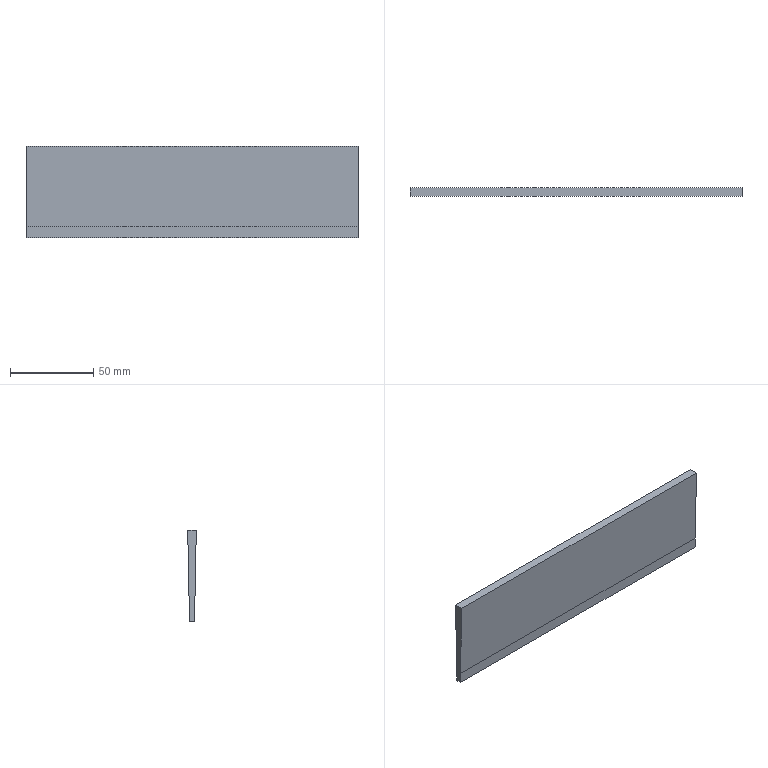Part | NX | features solid 2 | 1 solid | 8 faces | box 200 x 5.155 x 55.03 mm | volume 45049 mm3 | plane 8
STEP:
#1=CARTESIAN_POINT('',(-255.,2183.93,-987.43));
#2=VERTEX_POINT('',#1);
#3=CARTESIAN_POINT('',(-255.,2183.93,-980.8));
#4=VERTEX_POINT('',#3);
#5=CARTESIAN_POINT('',(-255.,2183.93,-987.43));
#6=DIRECTION('',(0.,0.,1.));
#7=VECTOR('',#6,1000.);
#8=LINE('',#5,#7);
#9=EDGE_CURVE('',#2,#4,#8,.T.);
#10=ORIENTED_EDGE('',*,*,#9,.T.);
#11=CARTESIAN_POINT('',(-55.,2183.93,-980.8));
#12=VERTEX_POINT('',#11);
#13=CARTESIAN_POINT('',(-55.,2183.93,-980.8));
#14=DIRECTION('',(-1.,0.,0.));
#15=VECTOR('',#14,1000.);
#16=LINE('',#13,#15);
#17=EDGE_CURVE('',#12,#4,#16,.T.);
#18=ORIENTED_EDGE('',*,*,#17,.F.);
#19=CARTESIAN_POINT('',(-55.,2183.93,-987.43));
#20=VERTEX_POINT('',#19);
#21=CARTESIAN_POINT('',(-55.,2183.93,-980.8));
#22=DIRECTION('',(0.,0.,-1.));
#23=VECTOR('',#22,1000.);
#24=LINE('',#21,#23);
#25=EDGE_CURVE('',#12,#20,#24,.T.);
#26=ORIENTED_EDGE('',*,*,#25,.T.);
#27=CARTESIAN_POINT('',(-55.,2183.93,-987.43));
#28=DIRECTION('',(-1.,0.,0.));
#29=VECTOR('',#28,1000.);
#30=LINE('',#27,#29);
#31=EDGE_CURVE('',#20,#2,#30,.T.);
#32=ORIENTED_EDGE('',*,*,#31,.T.);
#33=EDGE_LOOP('',(#10,#18,#26,#32));
#34=FACE_BOUND('',#33,.T.);
#35=CARTESIAN_POINT('',(-330.369,2183.93,-980.8));
#36=DIRECTION('',(0.,1.,0.));
#37=DIRECTION('',(-1.,0.,0.));
#38=AXIS2_PLACEMENT_3D('',#35,#36,#37);
#39=PLANE('',#38);
#40=ADVANCED_FACE('',(#34),#39,.T.);
#41=CARTESIAN_POINT('',(-255.,2180.67,-987.43));
#42=VERTEX_POINT('',#41);
#43=CARTESIAN_POINT('',(-255.,2180.67,-987.43));
#44=DIRECTION('',(0.,1.,0.));
#45=VECTOR('',#44,1000.);
#46=LINE('',#43,#45);
#47=EDGE_CURVE('',#42,#2,#46,.T.);
#48=ORIENTED_EDGE('',*,*,#47,.T.);
#49=ORIENTED_EDGE('',*,*,#31,.F.);
#50=CARTESIAN_POINT('',(-55.,2180.67,-987.43));
#51=VERTEX_POINT('',#50);
#52=CARTESIAN_POINT('',(-55.,2183.93,-987.43));
#53=DIRECTION('',(0.,-1.,0.));
#54=VECTOR('',#53,1000.);
#55=LINE('',#52,#54);
#56=EDGE_CURVE('',#20,#51,#55,.T.);
#57=ORIENTED_EDGE('',*,*,#56,.T.);
#58=CARTESIAN_POINT('',(-55.,2180.67,-987.43));
#59=DIRECTION('',(-1.,0.,0.));
#60=VECTOR('',#59,1000.);
#61=LINE('',#58,#60);
#62=EDGE_CURVE('',#51,#42,#61,.T.);
#63=ORIENTED_EDGE('',*,*,#62,.T.);
#64=EDGE_LOOP('',(#48,#49,#57,#63));
#65=FACE_BOUND('',#64,.T.);
#66=CARTESIAN_POINT('',(-330.369,2183.93,-987.43));
#67=DIRECTION('',(0.,0.,-1.));
#68=DIRECTION('',(-1.,0.,0.));
#69=AXIS2_PLACEMENT_3D('',#66,#67,#68);
#70=PLANE('',#69);
#71=ADVANCED_FACE('',(#65),#70,.T.);
#72=CARTESIAN_POINT('',(-255.,2180.67,-980.8));
#73=VERTEX_POINT('',#72);
#74=CARTESIAN_POINT('',(-255.,2180.67,-980.8));
#75=DIRECTION('',(0.,0.,-1.));
#76=VECTOR('',#75,1000.);
#77=LINE('',#74,#76);
#78=EDGE_CURVE('',#73,#42,#77,.T.);
#79=ORIENTED_EDGE('',*,*,#78,.T.);
#80=ORIENTED_EDGE('',*,*,#62,.F.);
#81=CARTESIAN_POINT('',(-55.,2180.67,-980.8));
#82=VERTEX_POINT('',#81);
#83=CARTESIAN_POINT('',(-55.,2180.67,-987.43));
#84=DIRECTION('',(0.,0.,1.));
#85=VECTOR('',#84,1000.);
#86=LINE('',#83,#85);
#87=EDGE_CURVE('',#51,#82,#86,.T.);
#88=ORIENTED_EDGE('',*,*,#87,.T.);
#89=CARTESIAN_POINT('',(-55.,2180.67,-980.8));
#90=DIRECTION('',(-1.,0.,0.));
#91=VECTOR('',#90,1000.);
#92=LINE('',#89,#91);
#93=EDGE_CURVE('',#82,#73,#92,.T.);
#94=ORIENTED_EDGE('',*,*,#93,.T.);
#95=EDGE_LOOP('',(#79,#80,#88,#94));
#96=FACE_BOUND('',#95,.T.);
#97=CARTESIAN_POINT('',(-330.369,2180.67,-985.93));
#98=DIRECTION('',(0.,-1.,0.));
#99=DIRECTION('',(0.,0.,1.));
#100=AXIS2_PLACEMENT_3D('',#97,#98,#99);
#101=PLANE('',#100);
#102=ADVANCED_FACE('',(#96),#101,.T.);
#103=ORIENTED_EDGE('',*,*,#93,.F.);
#104=CARTESIAN_POINT('',(-55.,2179.723,-932.4));
#105=VERTEX_POINT('',#104);
#106=CARTESIAN_POINT('',(-55.,2180.67,-980.8));
#107=DIRECTION('',(0.,-0.01957,0.9998));
#108=VECTOR('',#107,1000.);
#109=LINE('',#106,#108);
#110=EDGE_CURVE('',#82,#105,#109,.T.);
#111=ORIENTED_EDGE('',*,*,#110,.T.);
#112=CARTESIAN_POINT('',(-255.,2179.723,-932.4));
#113=VERTEX_POINT('',#112);
#114=CARTESIAN_POINT('',(-55.,2179.723,-932.4));
#115=DIRECTION('',(-1.,0.,0.));
#116=VECTOR('',#115,1000.);
#117=LINE('',#114,#116);
#118=EDGE_CURVE('',#105,#113,#117,.T.);
#119=ORIENTED_EDGE('',*,*,#118,.T.);
#120=CARTESIAN_POINT('',(-255.,2179.723,-932.4));
#121=DIRECTION('',(0.,0.01957,-0.9998));
#122=VECTOR('',#121,1000.);
#123=LINE('',#120,#122);
#124=EDGE_CURVE('',#113,#73,#123,.T.);
#125=ORIENTED_EDGE('',*,*,#124,.T.);
#126=EDGE_LOOP('',(#103,#111,#119,#125));
#127=FACE_BOUND('',#126,.T.);
#128=CARTESIAN_POINT('',(-330.369,2180.67,-980.8));
#129=DIRECTION('',(0.,-0.9998,-0.01957));
#130=DIRECTION('',(0.,-0.01957,0.9998));
#131=AXIS2_PLACEMENT_3D('',#128,#129,#130);
#132=PLANE('',#131);
#133=ADVANCED_FACE('',(#127),#132,.T.);
#134=ORIENTED_EDGE('',*,*,#9,.F.);
#135=ORIENTED_EDGE('',*,*,#47,.F.);
#136=ORIENTED_EDGE('',*,*,#78,.F.);
#137=ORIENTED_EDGE('',*,*,#124,.F.);
#138=CARTESIAN_POINT('',(-255.,2184.877,-932.4));
#139=VERTEX_POINT('',#138);
#140=CARTESIAN_POINT('',(-255.,2184.877,-932.4));
#141=DIRECTION('',(0.,-1.,0.));
#142=VECTOR('',#141,1000.);
#143=LINE('',#140,#142);
#144=EDGE_CURVE('',#139,#113,#143,.T.);
#145=ORIENTED_EDGE('',*,*,#144,.F.);
#146=CARTESIAN_POINT('',(-255.,2183.93,-980.8));
#147=DIRECTION('',(0.,0.01957,0.9998));
#148=VECTOR('',#147,1000.);
#149=LINE('',#146,#148);
#150=EDGE_CURVE('',#4,#139,#149,.T.);
#151=ORIENTED_EDGE('',*,*,#150,.F.);
#152=EDGE_LOOP('',(#134,#135,#136,#137,#145,#151));
#153=FACE_BOUND('',#152,.T.);
#154=CARTESIAN_POINT('',(-255.,2182.3,-987.8));
#155=DIRECTION('',(-1.,0.,0.));
#156=DIRECTION('',(0.,-1.,0.));
#157=AXIS2_PLACEMENT_3D('',#154,#155,#156);
#158=PLANE('',#157);
#159=ADVANCED_FACE('',(#153),#158,.T.);
#160=CARTESIAN_POINT('',(-55.,2184.877,-932.4));
#161=VERTEX_POINT('',#160);
#162=CARTESIAN_POINT('',(-55.,2184.877,-932.4));
#163=DIRECTION('',(-1.,0.,0.));
#164=VECTOR('',#163,1000.);
#165=LINE('',#162,#164);
#166=EDGE_CURVE('',#161,#139,#165,.T.);
#167=ORIENTED_EDGE('',*,*,#166,.F.);
#168=CARTESIAN_POINT('',(-55.,2184.877,-932.4));
#169=DIRECTION('',(0.,-0.01957,-0.9998));
#170=VECTOR('',#169,1000.);
#171=LINE('',#168,#170);
#172=EDGE_CURVE('',#161,#12,#171,.T.);
#173=ORIENTED_EDGE('',*,*,#172,.T.);
#174=ORIENTED_EDGE('',*,*,#17,.T.);
#175=ORIENTED_EDGE('',*,*,#150,.T.);
#176=EDGE_LOOP('',(#167,#173,#174,#175));
#177=FACE_BOUND('',#176,.T.);
#178=CARTESIAN_POINT('',(-330.369,2185.3,-910.8));
#179=DIRECTION('',(0.,0.9998,-0.01957));
#180=DIRECTION('',(0.,-0.01957,-0.9998));
#181=AXIS2_PLACEMENT_3D('',#178,#179,#180);
#182=PLANE('',#181);
#183=ADVANCED_FACE('',(#177),#182,.T.);
#184=ORIENTED_EDGE('',*,*,#87,.F.);
#185=ORIENTED_EDGE('',*,*,#56,.F.);
#186=ORIENTED_EDGE('',*,*,#25,.F.);
#187=ORIENTED_EDGE('',*,*,#172,.F.);
#188=CARTESIAN_POINT('',(-55.,2179.723,-932.4));
#189=DIRECTION('',(0.,1.,0.));
#190=VECTOR('',#189,1000.);
#191=LINE('',#188,#190);
#192=EDGE_CURVE('',#105,#161,#191,.T.);
#193=ORIENTED_EDGE('',*,*,#192,.F.);
#194=ORIENTED_EDGE('',*,*,#110,.F.);
#195=EDGE_LOOP('',(#184,#185,#186,#187,#193,#194));
#196=FACE_BOUND('',#195,.T.);
#197=CARTESIAN_POINT('',(-55.,2182.3,-987.8));
#198=DIRECTION('',(1.,0.,0.));
#199=DIRECTION('',(0.,1.,0.));
#200=AXIS2_PLACEMENT_3D('',#197,#198,#199);
#201=PLANE('',#200);
#202=ADVANCED_FACE('',(#196),#201,.T.);
#203=ORIENTED_EDGE('',*,*,#192,.T.);
#204=ORIENTED_EDGE('',*,*,#166,.T.);
#205=ORIENTED_EDGE('',*,*,#144,.T.);
#206=ORIENTED_EDGE('',*,*,#118,.F.);
#207=EDGE_LOOP('',(#203,#204,#205,#206));
#208=FACE_BOUND('',#207,.T.);
#209=CARTESIAN_POINT('',(-180.,2182.3,-932.4));
#210=DIRECTION('',(0.,0.,1.));
#211=DIRECTION('',(0.,1.,0.));
#212=AXIS2_PLACEMENT_3D('',#209,#210,#211);
#213=PLANE('',#212);
#214=ADVANCED_FACE('',(#208),#213,.T.);
#215=CLOSED_SHELL('',(#40,#71,#102,#133,#159,#183,#202,#214));
#216=MANIFOLD_SOLID_BREP('',#215);
#217=(LENGTH_UNIT()NAMED_UNIT(*)SI_UNIT(.MILLI.,.METRE.));
#218=UNCERTAINTY_MEASURE_WITH_UNIT(LENGTH_MEASURE(0.00001),#217,'','');
#219=(NAMED_UNIT(*)PLANE_ANGLE_UNIT()SI_UNIT($,.RADIAN.));
#220=(NAMED_UNIT(*)SI_UNIT($,.STERADIAN.)SOLID_ANGLE_UNIT());
#221=(GEOMETRIC_REPRESENTATION_CONTEXT(3)GLOBAL_UNCERTAINTY_ASSIGNED_CONTEXT((#218))GLOBAL_UNIT_ASSIGNED_CONTEXT((#217,#219,#220))REPRESENTATION_CONTEXT('',''));
#222=ADVANCED_BREP_SHAPE_REPRESENTATION('',(#216),#221);